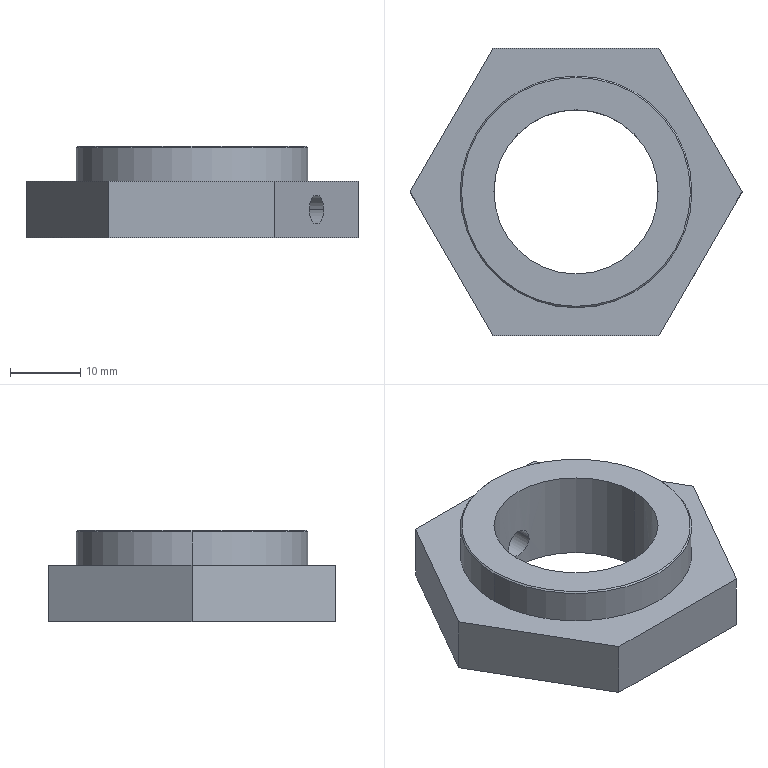Part | STEP file | BKN61-M25 | 1 solid | 19 faces | box 47.3 x 40.963 x 13 mm | volume 10083 mm3 | plane 9 | cylinder 8 | cone 2 | commonest cylinder face diameters 4.134 x4 23.376 x2 33 x2